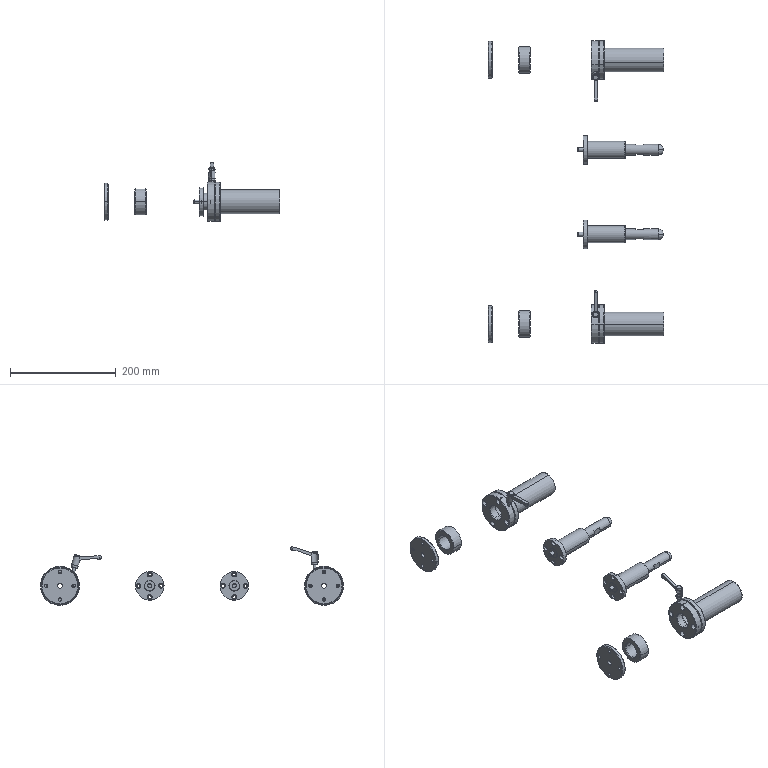Part | NX | features BREP 10 | 14 solids | 456 faces | box 333 x 574 x 111.263 mm | volume 683514 mm3 | cylinder 196 | plane 128 | torus 64 | cone 60 | sphere 8 | commonest cylinder face diameters 6.6 x32 9 x20 5.5 x16 6.4 x16 11 x16 8.5 x12